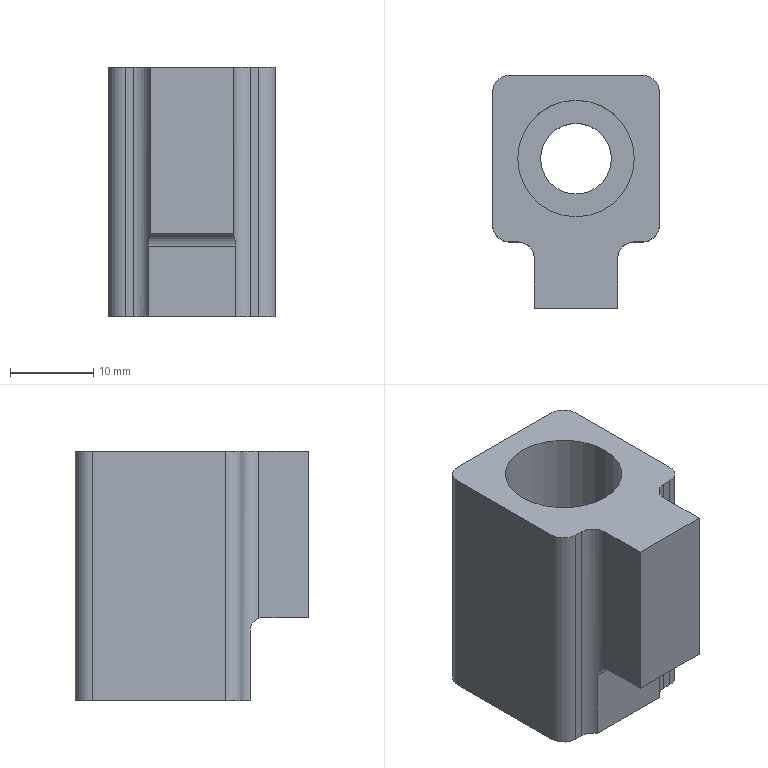Part | NX | features 1605030666 2 | 1 solid | 22 faces | box 20 x 28 x 30 mm | volume 10977 mm3 | plane 13 | cylinder 9 | commonest cylinder face diameters 4 x6 3 x1 8.5 x1 14 x1
STEP:
#1=CARTESIAN_POINT('',(-255.268,122.2,-31.5));
#2=VERTEX_POINT('',#1);
#3=CARTESIAN_POINT('',(-255.268,122.2,-23.));
#4=VERTEX_POINT('',#3);
#5=CARTESIAN_POINT('',(-255.268,122.2,-9.5));
#6=DIRECTION('',(0.,0.,-1.));
#7=VECTOR('',#6,1000.);
#8=LINE('',#5,#7);
#9=EDGE_CURVE('',#2,#4,#8,.F.);
#10=ORIENTED_EDGE('',*,*,#9,.F.);
#11=CARTESIAN_POINT('',(-244.732,122.2,-31.5));
#12=VERTEX_POINT('',#11);
#13=CARTESIAN_POINT('',(40.,122.2,-31.5));
#14=DIRECTION('',(-1.,0.,0.));
#15=VECTOR('',#14,1000.);
#16=LINE('',#13,#15);
#17=EDGE_CURVE('',#2,#12,#16,.F.);
#18=ORIENTED_EDGE('',*,*,#17,.T.);
#19=CARTESIAN_POINT('',(-244.732,122.2,-23.));
#20=VERTEX_POINT('',#19);
#21=CARTESIAN_POINT('',(-244.732,122.2,-1.5));
#22=DIRECTION('',(0.,0.,-1.));
#23=VECTOR('',#22,1000.);
#24=LINE('',#21,#23);
#25=EDGE_CURVE('',#20,#12,#24,.T.);
#26=ORIENTED_EDGE('',*,*,#25,.F.);
#27=CARTESIAN_POINT('',(-250.,122.2,-23.));
#28=DIRECTION('',(-1.,0.,0.));
#29=VECTOR('',#28,1000.);
#30=LINE('',#27,#29);
#31=EDGE_CURVE('',#4,#20,#30,.F.);
#32=ORIENTED_EDGE('',*,*,#31,.F.);
#33=EDGE_LOOP('',(#10,#18,#26,#32));
#34=FACE_BOUND('',#33,.T.);
#35=CARTESIAN_POINT('',(-250.,122.2,-76.5));
#36=DIRECTION('',(0.,1.,0.));
#37=DIRECTION('',(0.,0.,-1.));
#38=AXIS2_PLACEMENT_3D('',#35,#36,#37);
#39=PLANE('',#38);
#40=ADVANCED_FACE('',(#34),#39,.F.);
#41=ORIENTED_EDGE('',*,*,#17,.F.);
#42=CARTESIAN_POINT('',(-257.,123.2,-31.5));
#43=VERTEX_POINT('',#42);
#44=CARTESIAN_POINT('',(-257.,121.2,-31.5));
#45=DIRECTION('',(0.,0.,1.));
#46=DIRECTION('',(-1.,0.,0.));
#47=AXIS2_PLACEMENT_3D('',#44,#45,#46);
#48=CIRCLE('',#47,2.);
#49=EDGE_CURVE('',#43,#2,#48,.F.);
#50=ORIENTED_EDGE('',*,*,#49,.F.);
#51=CARTESIAN_POINT('',(-258.,123.2,-31.5));
#52=VERTEX_POINT('',#51);
#53=CARTESIAN_POINT('',(-256.,123.2,-31.5));
#54=DIRECTION('',(-1.,0.,0.));
#55=VECTOR('',#54,1000.);
#56=LINE('',#53,#55);
#57=EDGE_CURVE('',#43,#52,#56,.T.);
#58=ORIENTED_EDGE('',*,*,#57,.T.);
#59=CARTESIAN_POINT('',(-260.,125.2,-31.5));
#60=VERTEX_POINT('',#59);
#61=CARTESIAN_POINT('',(-258.,125.2,-31.5));
#62=DIRECTION('',(0.,0.,1.));
#63=DIRECTION('',(-1.,0.,0.));
#64=AXIS2_PLACEMENT_3D('',#61,#62,#63);
#65=CIRCLE('',#64,2.);
#66=EDGE_CURVE('',#60,#52,#65,.T.);
#67=ORIENTED_EDGE('',*,*,#66,.F.);
#68=CARTESIAN_POINT('',(-260.,141.2,-31.5));
#69=VERTEX_POINT('',#68);
#70=CARTESIAN_POINT('',(-260.,129.2,-31.5));
#71=DIRECTION('',(0.,1.,0.));
#72=VECTOR('',#71,1000.);
#73=LINE('',#70,#72);
#74=EDGE_CURVE('',#60,#69,#73,.T.);
#75=ORIENTED_EDGE('',*,*,#74,.T.);
#76=CARTESIAN_POINT('',(-258.,143.2,-31.5));
#77=VERTEX_POINT('',#76);
#78=CARTESIAN_POINT('',(-258.,141.2,-31.5));
#79=DIRECTION('',(0.,0.,1.));
#80=DIRECTION('',(-1.,0.,0.));
#81=AXIS2_PLACEMENT_3D('',#78,#79,#80);
#82=CIRCLE('',#81,2.);
#83=EDGE_CURVE('',#77,#69,#82,.T.);
#84=ORIENTED_EDGE('',*,*,#83,.F.);
#85=CARTESIAN_POINT('',(-242.,143.2,-31.5));
#86=VERTEX_POINT('',#85);
#87=CARTESIAN_POINT('',(-256.,143.2,-31.5));
#88=DIRECTION('',(1.,0.,0.));
#89=VECTOR('',#88,1000.);
#90=LINE('',#87,#89);
#91=EDGE_CURVE('',#77,#86,#90,.T.);
#92=ORIENTED_EDGE('',*,*,#91,.T.);
#93=CARTESIAN_POINT('',(-240.,141.2,-31.5));
#94=VERTEX_POINT('',#93);
#95=CARTESIAN_POINT('',(-242.,141.2,-31.5));
#96=DIRECTION('',(0.,0.,1.));
#97=DIRECTION('',(-1.,0.,0.));
#98=AXIS2_PLACEMENT_3D('',#95,#96,#97);
#99=CIRCLE('',#98,2.);
#100=EDGE_CURVE('',#94,#86,#99,.T.);
#101=ORIENTED_EDGE('',*,*,#100,.F.);
#102=CARTESIAN_POINT('',(-240.,125.2,-31.5));
#103=VERTEX_POINT('',#102);
#104=CARTESIAN_POINT('',(-240.,129.2,-31.5));
#105=DIRECTION('',(0.,-1.,0.));
#106=VECTOR('',#105,1000.);
#107=LINE('',#104,#106);
#108=EDGE_CURVE('',#94,#103,#107,.T.);
#109=ORIENTED_EDGE('',*,*,#108,.T.);
#110=CARTESIAN_POINT('',(-242.,123.2,-31.5));
#111=VERTEX_POINT('',#110);
#112=CARTESIAN_POINT('',(-242.,125.2,-31.5));
#113=DIRECTION('',(0.,0.,1.));
#114=DIRECTION('',(-1.,0.,0.));
#115=AXIS2_PLACEMENT_3D('',#112,#113,#114);
#116=CIRCLE('',#115,2.);
#117=EDGE_CURVE('',#111,#103,#116,.T.);
#118=ORIENTED_EDGE('',*,*,#117,.F.);
#119=CARTESIAN_POINT('',(-243.,123.2,-31.5));
#120=VERTEX_POINT('',#119);
#121=CARTESIAN_POINT('',(-256.,123.2,-31.5));
#122=DIRECTION('',(-1.,0.,0.));
#123=VECTOR('',#122,1000.);
#124=LINE('',#121,#123);
#125=EDGE_CURVE('',#111,#120,#124,.T.);
#126=ORIENTED_EDGE('',*,*,#125,.T.);
#127=CARTESIAN_POINT('',(-243.,121.2,-31.5));
#128=DIRECTION('',(0.,0.,1.));
#129=DIRECTION('',(-1.,0.,0.));
#130=AXIS2_PLACEMENT_3D('',#127,#128,#129);
#131=CIRCLE('',#130,2.);
#132=EDGE_CURVE('',#12,#120,#131,.F.);
#133=ORIENTED_EDGE('',*,*,#132,.F.);
#134=EDGE_LOOP('',(#41,#50,#58,#67,#75,#84,#92,#101,#109,#118,#126,#133));
#135=FACE_BOUND('',#134,.T.);
#136=CARTESIAN_POINT('',(-254.25,133.2,-31.5));
#137=VERTEX_POINT('',#136);
#138=CARTESIAN_POINT('',(-250.,133.2,-31.5));
#139=DIRECTION('',(0.,0.,-1.));
#140=DIRECTION('',(-1.,0.,0.));
#141=AXIS2_PLACEMENT_3D('',#138,#139,#140);
#142=CIRCLE('',#141,4.25);
#143=EDGE_CURVE('',#137,#137,#142,.T.);
#144=ORIENTED_EDGE('',*,*,#143,.F.);
#145=EDGE_LOOP('',(#144));
#146=FACE_BOUND('',#145,.T.);
#147=CARTESIAN_POINT('',(40.,31.936,-31.5));
#148=DIRECTION('',(0.,0.,-1.));
#149=DIRECTION('',(-1.,0.,0.));
#150=AXIS2_PLACEMENT_3D('',#147,#148,#149);
#151=PLANE('',#150);
#152=ADVANCED_FACE('',(#135,#146),#151,.T.);
#153=CARTESIAN_POINT('',(-243.,123.2,-1.5));
#154=VERTEX_POINT('',#153);
#155=CARTESIAN_POINT('',(-245.,121.2,-1.5));
#156=VERTEX_POINT('',#155);
#157=CARTESIAN_POINT('',(-243.,121.2,-1.5));
#158=DIRECTION('',(0.,0.,-1.));
#159=DIRECTION('',(1.,0.,0.));
#160=AXIS2_PLACEMENT_3D('',#157,#158,#159);
#161=CIRCLE('',#160,2.);
#162=EDGE_CURVE('',#154,#156,#161,.F.);
#163=ORIENTED_EDGE('',*,*,#162,.F.);
#164=CARTESIAN_POINT('',(-242.,123.2,-1.5));
#165=VERTEX_POINT('',#164);
#166=CARTESIAN_POINT('',(-256.,123.2,-1.5));
#167=DIRECTION('',(1.,0.,0.));
#168=VECTOR('',#167,1000.);
#169=LINE('',#166,#168);
#170=EDGE_CURVE('',#154,#165,#169,.T.);
#171=ORIENTED_EDGE('',*,*,#170,.T.);
#172=CARTESIAN_POINT('',(-240.,125.2,-1.5));
#173=VERTEX_POINT('',#172);
#174=CARTESIAN_POINT('',(-242.,125.2,-1.5));
#175=DIRECTION('',(0.,0.,-1.));
#176=DIRECTION('',(1.,0.,0.));
#177=AXIS2_PLACEMENT_3D('',#174,#175,#176);
#178=CIRCLE('',#177,2.);
#179=EDGE_CURVE('',#173,#165,#178,.T.);
#180=ORIENTED_EDGE('',*,*,#179,.F.);
#181=CARTESIAN_POINT('',(-240.,141.2,-1.5));
#182=VERTEX_POINT('',#181);
#183=CARTESIAN_POINT('',(-240.,129.2,-1.5));
#184=DIRECTION('',(0.,1.,0.));
#185=VECTOR('',#184,1000.);
#186=LINE('',#183,#185);
#187=EDGE_CURVE('',#173,#182,#186,.T.);
#188=ORIENTED_EDGE('',*,*,#187,.T.);
#189=CARTESIAN_POINT('',(-242.,143.2,-1.5));
#190=VERTEX_POINT('',#189);
#191=CARTESIAN_POINT('',(-242.,141.2,-1.5));
#192=DIRECTION('',(0.,0.,-1.));
#193=DIRECTION('',(1.,0.,0.));
#194=AXIS2_PLACEMENT_3D('',#191,#192,#193);
#195=CIRCLE('',#194,2.);
#196=EDGE_CURVE('',#190,#182,#195,.T.);
#197=ORIENTED_EDGE('',*,*,#196,.F.);
#198=CARTESIAN_POINT('',(-258.,143.2,-1.5));
#199=VERTEX_POINT('',#198);
#200=CARTESIAN_POINT('',(-256.,143.2,-1.5));
#201=DIRECTION('',(-1.,0.,0.));
#202=VECTOR('',#201,1000.);
#203=LINE('',#200,#202);
#204=EDGE_CURVE('',#190,#199,#203,.T.);
#205=ORIENTED_EDGE('',*,*,#204,.T.);
#206=CARTESIAN_POINT('',(-260.,141.2,-1.5));
#207=VERTEX_POINT('',#206);
#208=CARTESIAN_POINT('',(-258.,141.2,-1.5));
#209=DIRECTION('',(0.,0.,-1.));
#210=DIRECTION('',(1.,0.,0.));
#211=AXIS2_PLACEMENT_3D('',#208,#209,#210);
#212=CIRCLE('',#211,2.);
#213=EDGE_CURVE('',#207,#199,#212,.T.);
#214=ORIENTED_EDGE('',*,*,#213,.F.);
#215=CARTESIAN_POINT('',(-260.,125.2,-1.5));
#216=VERTEX_POINT('',#215);
#217=CARTESIAN_POINT('',(-260.,129.2,-1.5));
#218=DIRECTION('',(0.,-1.,0.));
#219=VECTOR('',#218,1000.);
#220=LINE('',#217,#219);
#221=EDGE_CURVE('',#207,#216,#220,.T.);
#222=ORIENTED_EDGE('',*,*,#221,.T.);
#223=CARTESIAN_POINT('',(-258.,123.2,-1.5));
#224=VERTEX_POINT('',#223);
#225=CARTESIAN_POINT('',(-258.,125.2,-1.5));
#226=DIRECTION('',(0.,0.,-1.));
#227=DIRECTION('',(1.,0.,0.));
#228=AXIS2_PLACEMENT_3D('',#225,#226,#227);
#229=CIRCLE('',#228,2.);
#230=EDGE_CURVE('',#224,#216,#229,.T.);
#231=ORIENTED_EDGE('',*,*,#230,.F.);
#232=CARTESIAN_POINT('',(-257.,123.2,-1.5));
#233=VERTEX_POINT('',#232);
#234=CARTESIAN_POINT('',(-256.,123.2,-1.5));
#235=DIRECTION('',(1.,0.,0.));
#236=VECTOR('',#235,1000.);
#237=LINE('',#234,#236);
#238=EDGE_CURVE('',#224,#233,#237,.T.);
#239=ORIENTED_EDGE('',*,*,#238,.T.);
#240=CARTESIAN_POINT('',(-255.,121.2,-1.5));
#241=VERTEX_POINT('',#240);
#242=CARTESIAN_POINT('',(-257.,121.2,-1.5));
#243=DIRECTION('',(0.,0.,-1.));
#244=DIRECTION('',(1.,0.,0.));
#245=AXIS2_PLACEMENT_3D('',#242,#243,#244);
#246=CIRCLE('',#245,2.);
#247=EDGE_CURVE('',#241,#233,#246,.F.);
#248=ORIENTED_EDGE('',*,*,#247,.F.);
#249=CARTESIAN_POINT('',(-255.,115.2,-1.5));
#250=VERTEX_POINT('',#249);
#251=CARTESIAN_POINT('',(-255.,117.7,-1.5));
#252=DIRECTION('',(0.,-1.,0.));
#253=VECTOR('',#252,1000.);
#254=LINE('',#251,#253);
#255=EDGE_CURVE('',#241,#250,#254,.T.);
#256=ORIENTED_EDGE('',*,*,#255,.T.);
#257=CARTESIAN_POINT('',(-245.,115.2,-1.5));
#258=VERTEX_POINT('',#257);
#259=CARTESIAN_POINT('',(-250.,115.2,-1.5));
#260=DIRECTION('',(1.,0.,0.));
#261=VECTOR('',#260,1000.);
#262=LINE('',#259,#261);
#263=EDGE_CURVE('',#250,#258,#262,.T.);
#264=ORIENTED_EDGE('',*,*,#263,.T.);
#265=CARTESIAN_POINT('',(-245.,117.7,-1.5));
#266=DIRECTION('',(0.,1.,0.));
#267=VECTOR('',#266,1000.);
#268=LINE('',#265,#267);
#269=EDGE_CURVE('',#258,#156,#268,.T.);
#270=ORIENTED_EDGE('',*,*,#269,.T.);
#271=EDGE_LOOP('',(#163,#171,#180,#188,#197,#205,#214,#222,#231,#239,#248,#256,#264,#270));
#272=FACE_BOUND('',#271,.T.);
#273=CARTESIAN_POINT('',(-243.,133.2,-1.5));
#274=VERTEX_POINT('',#273);
#275=CARTESIAN_POINT('',(-250.,133.2,-1.5));
#276=DIRECTION('',(0.,0.,1.));
#277=DIRECTION('',(1.,0.,0.));
#278=AXIS2_PLACEMENT_3D('',#275,#276,#277);
#279=CIRCLE('',#278,7.);
#280=EDGE_CURVE('',#274,#274,#279,.F.);
#281=ORIENTED_EDGE('',*,*,#280,.T.);
#282=EDGE_LOOP('',(#281));
#283=FACE_BOUND('',#282,.T.);
#284=CARTESIAN_POINT('',(-250.,117.7,-1.5));
#285=DIRECTION('',(0.,0.,1.));
#286=DIRECTION('',(1.,0.,0.));
#287=AXIS2_PLACEMENT_3D('',#284,#285,#286);
#288=PLANE('',#287);
#289=ADVANCED_FACE('',(#272,#283),#288,.T.);
#290=ORIENTED_EDGE('',*,*,#238,.F.);
#291=CARTESIAN_POINT('',(-258.,123.2,-1.5));
#292=DIRECTION('',(0.,0.,-1.));
#293=VECTOR('',#292,1000.);
#294=LINE('',#291,#293);
#295=EDGE_CURVE('',#52,#224,#294,.F.);
#296=ORIENTED_EDGE('',*,*,#295,.F.);
#297=ORIENTED_EDGE('',*,*,#57,.F.);
#298=CARTESIAN_POINT('',(-257.,123.2,-36.5));
#299=DIRECTION('',(0.,0.,1.));
#300=VECTOR('',#299,1000.);
#301=LINE('',#298,#300);
#302=EDGE_CURVE('',#233,#43,#301,.F.);
#303=ORIENTED_EDGE('',*,*,#302,.F.);
#304=EDGE_LOOP('',(#290,#296,#297,#303));
#305=FACE_BOUND('',#304,.T.);
#306=CARTESIAN_POINT('',(-256.,123.2,-1.5));
#307=DIRECTION('',(0.,-1.,0.));
#308=DIRECTION('',(0.,0.,1.));
#309=AXIS2_PLACEMENT_3D('',#306,#307,#308);
#310=PLANE('',#309);
#311=ADVANCED_FACE('',(#305),#310,.T.);
#312=ORIENTED_EDGE('',*,*,#91,.F.);
#313=CARTESIAN_POINT('',(-258.,143.2,-1.5));
#314=DIRECTION('',(0.,0.,-1.));
#315=VECTOR('',#314,1000.);
#316=LINE('',#313,#315);
#317=EDGE_CURVE('',#199,#77,#316,.T.);
#318=ORIENTED_EDGE('',*,*,#317,.F.);
#319=ORIENTED_EDGE('',*,*,#204,.F.);
#320=CARTESIAN_POINT('',(-242.,143.2,-1.5));
#321=DIRECTION('',(0.,0.,-1.));
#322=VECTOR('',#321,1000.);
#323=LINE('',#320,#322);
#324=EDGE_CURVE('',#86,#190,#323,.F.);
#325=ORIENTED_EDGE('',*,*,#324,.F.);
#326=EDGE_LOOP('',(#312,#318,#319,#325));
#327=FACE_BOUND('',#326,.T.);
#328=CARTESIAN_POINT('',(-256.,143.2,-1.5));
#329=DIRECTION('',(0.,1.,0.));
#330=DIRECTION('',(0.,0.,-1.));
#331=AXIS2_PLACEMENT_3D('',#328,#329,#330);
#332=PLANE('',#331);
#333=ADVANCED_FACE('',(#327),#332,.T.);
#334=ORIENTED_EDGE('',*,*,#108,.F.);
#335=CARTESIAN_POINT('',(-240.,141.2,-1.5));
#336=DIRECTION('',(0.,0.,-1.));
#337=VECTOR('',#336,1000.);
#338=LINE('',#335,#337);
#339=EDGE_CURVE('',#182,#94,#338,.T.);
#340=ORIENTED_EDGE('',*,*,#339,.F.);
#341=ORIENTED_EDGE('',*,*,#187,.F.);
#342=CARTESIAN_POINT('',(-240.,125.2,-1.5));
#343=DIRECTION('',(0.,0.,-1.));
#344=VECTOR('',#343,1000.);
#345=LINE('',#342,#344);
#346=EDGE_CURVE('',#103,#173,#345,.F.);
#347=ORIENTED_EDGE('',*,*,#346,.F.);
#348=EDGE_LOOP('',(#334,#340,#341,#347));
#349=FACE_BOUND('',#348,.T.);
#350=CARTESIAN_POINT('',(-240.,129.2,-1.5));
#351=DIRECTION('',(1.,0.,0.));
#352=DIRECTION('',(0.,0.,-1.));
#353=AXIS2_PLACEMENT_3D('',#350,#351,#352);
#354=PLANE('',#353);
#355=ADVANCED_FACE('',(#349),#354,.T.);
#356=ORIENTED_EDGE('',*,*,#125,.F.);
#357=CARTESIAN_POINT('',(-242.,123.2,-1.5));
#358=DIRECTION('',(0.,0.,-1.));
#359=VECTOR('',#358,1000.);
#360=LINE('',#357,#359);
#361=EDGE_CURVE('',#165,#111,#360,.T.);
#362=ORIENTED_EDGE('',*,*,#361,.F.);
#363=ORIENTED_EDGE('',*,*,#170,.F.);
#364=CARTESIAN_POINT('',(-243.,123.2,-1.5));
#365=DIRECTION('',(0.,0.,1.));
#366=VECTOR('',#365,1000.);
#367=LINE('',#364,#366);
#368=EDGE_CURVE('',#120,#154,#367,.T.);
#369=ORIENTED_EDGE('',*,*,#368,.F.);
#370=EDGE_LOOP('',(#356,#362,#363,#369));
#371=FACE_BOUND('',#370,.T.);
#372=CARTESIAN_POINT('',(-256.,123.2,-1.5));
#373=DIRECTION('',(0.,-1.,0.));
#374=DIRECTION('',(0.,0.,1.));
#375=AXIS2_PLACEMENT_3D('',#372,#373,#374);
#376=PLANE('',#375);
#377=ADVANCED_FACE('',(#371),#376,.T.);
#378=ORIENTED_EDGE('',*,*,#221,.F.);
#379=CARTESIAN_POINT('',(-260.,141.2,-1.5));
#380=DIRECTION('',(0.,0.,-1.));
#381=VECTOR('',#380,1000.);
#382=LINE('',#379,#381);
#383=EDGE_CURVE('',#69,#207,#382,.F.);
#384=ORIENTED_EDGE('',*,*,#383,.F.);
#385=ORIENTED_EDGE('',*,*,#74,.F.);
#386=CARTESIAN_POINT('',(-260.,125.2,-1.5));
#387=DIRECTION('',(0.,0.,-1.));
#388=VECTOR('',#387,1000.);
#389=LINE('',#386,#388);
#390=EDGE_CURVE('',#216,#60,#389,.T.);
#391=ORIENTED_EDGE('',*,*,#390,.F.);
#392=EDGE_LOOP('',(#378,#384,#385,#391));
#393=FACE_BOUND('',#392,.T.);
#394=CARTESIAN_POINT('',(-260.,129.2,-1.5));
#395=DIRECTION('',(-1.,0.,0.));
#396=DIRECTION('',(0.,0.,1.));
#397=AXIS2_PLACEMENT_3D('',#394,#395,#396);
#398=PLANE('',#397);
#399=ADVANCED_FACE('',(#393),#398,.T.);
#400=ORIENTED_EDGE('',*,*,#213,.T.);
#401=ORIENTED_EDGE('',*,*,#317,.T.);
#402=ORIENTED_EDGE('',*,*,#83,.T.);
#403=ORIENTED_EDGE('',*,*,#383,.T.);
#404=EDGE_LOOP('',(#400,#401,#402,#403));
#405=FACE_BOUND('',#404,.T.);
#406=CARTESIAN_POINT('',(-258.,141.2,-1.5));
#407=DIRECTION('',(0.,0.,-1.));
#408=DIRECTION('',(-1.,0.,0.));
#409=AXIS2_PLACEMENT_3D('',#406,#407,#408);
#410=CYLINDRICAL_SURFACE('',#409,2.);
#411=ADVANCED_FACE('',(#405),#410,.T.);
#412=ORIENTED_EDGE('',*,*,#196,.T.);
#413=ORIENTED_EDGE('',*,*,#339,.T.);
#414=ORIENTED_EDGE('',*,*,#100,.T.);
#415=ORIENTED_EDGE('',*,*,#324,.T.);
#416=EDGE_LOOP('',(#412,#413,#414,#415));
#417=FACE_BOUND('',#416,.T.);
#418=CARTESIAN_POINT('',(-242.,141.2,-1.5));
#419=DIRECTION('',(0.,0.,-1.));
#420=DIRECTION('',(-1.,0.,0.));
#421=AXIS2_PLACEMENT_3D('',#418,#419,#420);
#422=CYLINDRICAL_SURFACE('',#421,2.);
#423=ADVANCED_FACE('',(#417),#422,.T.);
#424=ORIENTED_EDGE('',*,*,#179,.T.);
#425=ORIENTED_EDGE('',*,*,#361,.T.);
#426=ORIENTED_EDGE('',*,*,#117,.T.);
#427=ORIENTED_EDGE('',*,*,#346,.T.);
#428=EDGE_LOOP('',(#424,#425,#426,#427));
#429=FACE_BOUND('',#428,.T.);
#430=CARTESIAN_POINT('',(-242.,125.2,-1.5));
#431=DIRECTION('',(0.,0.,-1.));
#432=DIRECTION('',(-1.,0.,0.));
#433=AXIS2_PLACEMENT_3D('',#430,#431,#432);
#434=CYLINDRICAL_SURFACE('',#433,2.);
#435=ADVANCED_FACE('',(#429),#434,.T.);
#436=ORIENTED_EDGE('',*,*,#230,.T.);
#437=ORIENTED_EDGE('',*,*,#390,.T.);
#438=ORIENTED_EDGE('',*,*,#66,.T.);
#439=ORIENTED_EDGE('',*,*,#295,.T.);
#440=EDGE_LOOP('',(#436,#437,#438,#439));
#441=FACE_BOUND('',#440,.T.);
#442=CARTESIAN_POINT('',(-258.,125.2,-1.5));
#443=DIRECTION('',(0.,0.,-1.));
#444=DIRECTION('',(-1.,0.,0.));
#445=AXIS2_PLACEMENT_3D('',#442,#443,#444);
#446=CYLINDRICAL_SURFACE('',#445,2.);
#447=ADVANCED_FACE('',(#441),#446,.T.);
#448=ORIENTED_EDGE('',*,*,#49,.T.);
#449=ORIENTED_EDGE('',*,*,#9,.T.);
#450=CARTESIAN_POINT('',(-255.,121.2,-21.586));
#451=VERTEX_POINT('',#450);
#452=CARTESIAN_POINT('',(-255.,121.2,-21.586));
#453=CARTESIAN_POINT('',(-255.,121.794,-21.796));
#454=CARTESIAN_POINT('',(-255.268,122.2,-22.37));
#455=CARTESIAN_POINT('',(-255.268,122.2,-23.));
#456=B_SPLINE_CURVE_WITH_KNOTS('',3,(#452,#453,#454,#455),.UNSPECIFIED.,.F.,.F.,(4,4),(0.,0.001858),.UNSPECIFIED.);
#457=EDGE_CURVE('',#451,#4,#456,.T.);
#458=ORIENTED_EDGE('',*,*,#457,.F.);
#459=CARTESIAN_POINT('',(-255.,121.2,-9.5));
#460=DIRECTION('',(0.,0.,-1.));
#461=VECTOR('',#460,1000.);
#462=LINE('',#459,#461);
#463=EDGE_CURVE('',#451,#241,#462,.F.);
#464=ORIENTED_EDGE('',*,*,#463,.T.);
#465=ORIENTED_EDGE('',*,*,#247,.T.);
#466=ORIENTED_EDGE('',*,*,#302,.T.);
#467=EDGE_LOOP('',(#448,#449,#458,#464,#465,#466));
#468=FACE_BOUND('',#467,.T.);
#469=CARTESIAN_POINT('',(-257.,121.2,-9.5));
#470=DIRECTION('',(0.,0.,-1.));
#471=DIRECTION('',(-1.,0.,0.));
#472=AXIS2_PLACEMENT_3D('',#469,#470,#471);
#473=CYLINDRICAL_SURFACE('',#472,2.);
#474=ADVANCED_FACE('',(#468),#473,.F.);
#475=ORIENTED_EDGE('',*,*,#132,.T.);
#476=ORIENTED_EDGE('',*,*,#368,.T.);
#477=ORIENTED_EDGE('',*,*,#162,.T.);
#478=CARTESIAN_POINT('',(-245.,121.2,-21.586));
#479=VERTEX_POINT('',#478);
#480=CARTESIAN_POINT('',(-245.,121.2,-36.5));
#481=DIRECTION('',(0.,0.,1.));
#482=VECTOR('',#481,1000.);
#483=LINE('',#480,#482);
#484=EDGE_CURVE('',#156,#479,#483,.F.);
#485=ORIENTED_EDGE('',*,*,#484,.T.);
#486=CARTESIAN_POINT('',(-244.732,122.2,-23.));
#487=CARTESIAN_POINT('',(-244.732,122.2,-22.37));
#488=CARTESIAN_POINT('',(-245.,121.794,-21.796));
#489=CARTESIAN_POINT('',(-245.,121.2,-21.586));
#490=B_SPLINE_CURVE_WITH_KNOTS('',3,(#486,#487,#488,#489),.UNSPECIFIED.,.F.,.F.,(4,4),(0.,0.001858),.UNSPECIFIED.);
#491=EDGE_CURVE('',#20,#479,#490,.T.);
#492=ORIENTED_EDGE('',*,*,#491,.F.);
#493=ORIENTED_EDGE('',*,*,#25,.T.);
#494=EDGE_LOOP('',(#475,#476,#477,#485,#492,#493));
#495=FACE_BOUND('',#494,.T.);
#496=CARTESIAN_POINT('',(-243.,121.2,-1.5));
#497=DIRECTION('',(0.,0.,-1.));
#498=DIRECTION('',(-1.,0.,0.));
#499=AXIS2_PLACEMENT_3D('',#496,#497,#498);
#500=CYLINDRICAL_SURFACE('',#499,2.);
#501=ADVANCED_FACE('',(#495),#500,.F.);
#502=CARTESIAN_POINT('',(-254.25,133.2,-11.5));
#503=VERTEX_POINT('',#502);
#504=CARTESIAN_POINT('',(-250.,133.2,-11.5));
#505=DIRECTION('',(0.,0.,-1.));
#506=DIRECTION('',(-1.,0.,0.));
#507=AXIS2_PLACEMENT_3D('',#504,#505,#506);
#508=CIRCLE('',#507,4.25);
#509=EDGE_CURVE('',#503,#503,#508,.T.);
#510=ORIENTED_EDGE('',*,*,#509,.F.);
#511=EDGE_LOOP('',(#510));
#512=FACE_BOUND('',#511,.T.);
#513=ORIENTED_EDGE('',*,*,#143,.T.);
#514=EDGE_LOOP('',(#513));
#515=FACE_BOUND('',#514,.T.);
#516=CARTESIAN_POINT('',(-250.,133.2,-31.5));
#517=DIRECTION('',(0.,0.,1.));
#518=DIRECTION('',(1.,0.,0.));
#519=AXIS2_PLACEMENT_3D('',#516,#517,#518);
#520=CYLINDRICAL_SURFACE('',#519,4.25);
#521=ADVANCED_FACE('',(#512,#515),#520,.F.);
#522=CARTESIAN_POINT('',(-257.,133.2,-11.5));
#523=VERTEX_POINT('',#522);
#524=CARTESIAN_POINT('',(-250.,133.2,-11.5));
#525=DIRECTION('',(0.,0.,-1.));
#526=DIRECTION('',(-1.,0.,0.));
#527=AXIS2_PLACEMENT_3D('',#524,#525,#526);
#528=CIRCLE('',#527,7.);
#529=EDGE_CURVE('',#523,#523,#528,.F.);
#530=ORIENTED_EDGE('',*,*,#529,.T.);
#531=EDGE_LOOP('',(#530));
#532=FACE_BOUND('',#531,.T.);
#533=ORIENTED_EDGE('',*,*,#509,.T.);
#534=EDGE_LOOP('',(#533));
#535=FACE_BOUND('',#534,.T.);
#536=CARTESIAN_POINT('',(-250.,133.2,-11.5));
#537=DIRECTION('',(0.,0.,-1.));
#538=DIRECTION('',(-1.,0.,0.));
#539=AXIS2_PLACEMENT_3D('',#536,#537,#538);
#540=PLANE('',#539);
#541=ADVANCED_FACE('',(#532,#535),#540,.F.);
#542=ORIENTED_EDGE('',*,*,#280,.F.);
#543=EDGE_LOOP('',(#542));
#544=FACE_BOUND('',#543,.T.);
#545=ORIENTED_EDGE('',*,*,#529,.F.);
#546=EDGE_LOOP('',(#545));
#547=FACE_BOUND('',#546,.T.);
#548=CARTESIAN_POINT('',(-250.,133.2,-11.5));
#549=DIRECTION('',(0.,0.,1.));
#550=DIRECTION('',(1.,0.,0.));
#551=AXIS2_PLACEMENT_3D('',#548,#549,#550);
#552=CYLINDRICAL_SURFACE('',#551,7.);
#553=ADVANCED_FACE('',(#544,#547),#552,.F.);
#554=CARTESIAN_POINT('',(-255.,115.2,-21.5));
#555=VERTEX_POINT('',#554);
#556=CARTESIAN_POINT('',(-255.,115.2,-9.5));
#557=DIRECTION('',(0.,0.,1.));
#558=VECTOR('',#557,1000.);
#559=LINE('',#556,#558);
#560=EDGE_CURVE('',#555,#250,#559,.T.);
#561=ORIENTED_EDGE('',*,*,#560,.F.);
#562=CARTESIAN_POINT('',(-245.,115.2,-21.5));
#563=VERTEX_POINT('',#562);
#564=CARTESIAN_POINT('',(-250.,115.2,-21.5));
#565=DIRECTION('',(-1.,0.,0.));
#566=VECTOR('',#565,1000.);
#567=LINE('',#564,#566);
#568=EDGE_CURVE('',#563,#555,#567,.T.);
#569=ORIENTED_EDGE('',*,*,#568,.F.);
#570=CARTESIAN_POINT('',(-245.,115.2,-9.5));
#571=DIRECTION('',(0.,0.,1.));
#572=VECTOR('',#571,1000.);
#573=LINE('',#570,#572);
#574=EDGE_CURVE('',#563,#258,#573,.T.);
#575=ORIENTED_EDGE('',*,*,#574,.T.);
#576=ORIENTED_EDGE('',*,*,#263,.F.);
#577=EDGE_LOOP('',(#561,#569,#575,#576));
#578=FACE_BOUND('',#577,.T.);
#579=CARTESIAN_POINT('',(-250.,115.2,-9.5));
#580=DIRECTION('',(0.,-1.,0.));
#581=DIRECTION('',(0.,0.,1.));
#582=AXIS2_PLACEMENT_3D('',#579,#580,#581);
#583=PLANE('',#582);
#584=ADVANCED_FACE('',(#578),#583,.T.);
#585=ORIENTED_EDGE('',*,*,#269,.F.);
#586=ORIENTED_EDGE('',*,*,#574,.F.);
#587=CARTESIAN_POINT('',(-245.,120.7,-21.5));
#588=VERTEX_POINT('',#587);
#589=CARTESIAN_POINT('',(-245.,117.7,-21.5));
#590=DIRECTION('',(0.,-1.,0.));
#591=VECTOR('',#590,1000.);
#592=LINE('',#589,#591);
#593=EDGE_CURVE('',#588,#563,#592,.T.);
#594=ORIENTED_EDGE('',*,*,#593,.F.);
#595=CARTESIAN_POINT('',(-245.,120.7,-23.));
#596=DIRECTION('',(-1.,0.,0.));
#597=DIRECTION('',(0.,0.,-1.));
#598=AXIS2_PLACEMENT_3D('',#595,#596,#597);
#599=CIRCLE('',#598,1.5);
#600=EDGE_CURVE('',#479,#588,#599,.F.);
#601=ORIENTED_EDGE('',*,*,#600,.F.);
#602=ORIENTED_EDGE('',*,*,#484,.F.);
#603=EDGE_LOOP('',(#585,#586,#594,#601,#602));
#604=FACE_BOUND('',#603,.T.);
#605=CARTESIAN_POINT('',(-245.,117.7,-9.5));
#606=DIRECTION('',(1.,0.,0.));
#607=DIRECTION('',(0.,0.,-1.));
#608=AXIS2_PLACEMENT_3D('',#605,#606,#607);
#609=PLANE('',#608);
#610=ADVANCED_FACE('',(#604),#609,.T.);
#611=CARTESIAN_POINT('',(-255.,120.7,-21.5));
#612=VERTEX_POINT('',#611);
#613=CARTESIAN_POINT('',(-255.,117.7,-21.5));
#614=DIRECTION('',(0.,1.,0.));
#615=VECTOR('',#614,1000.);
#616=LINE('',#613,#615);
#617=EDGE_CURVE('',#555,#612,#616,.T.);
#618=ORIENTED_EDGE('',*,*,#617,.F.);
#619=ORIENTED_EDGE('',*,*,#560,.T.);
#620=ORIENTED_EDGE('',*,*,#255,.F.);
#621=ORIENTED_EDGE('',*,*,#463,.F.);
#622=CARTESIAN_POINT('',(-255.,120.7,-23.));
#623=DIRECTION('',(1.,0.,0.));
#624=DIRECTION('',(0.,0.,1.));
#625=AXIS2_PLACEMENT_3D('',#622,#623,#624);
#626=CIRCLE('',#625,1.5);
#627=EDGE_CURVE('',#612,#451,#626,.F.);
#628=ORIENTED_EDGE('',*,*,#627,.F.);
#629=EDGE_LOOP('',(#618,#619,#620,#621,#628));
#630=FACE_BOUND('',#629,.T.);
#631=CARTESIAN_POINT('',(-255.,117.7,-9.5));
#632=DIRECTION('',(-1.,0.,0.));
#633=DIRECTION('',(0.,0.,1.));
#634=AXIS2_PLACEMENT_3D('',#631,#632,#633);
#635=PLANE('',#634);
#636=ADVANCED_FACE('',(#630),#635,.T.);
#637=ORIENTED_EDGE('',*,*,#593,.T.);
#638=ORIENTED_EDGE('',*,*,#568,.T.);
#639=ORIENTED_EDGE('',*,*,#617,.T.);
#640=CARTESIAN_POINT('',(40.,120.7,-21.5));
#641=DIRECTION('',(-1.,0.,0.));
#642=VECTOR('',#641,1000.);
#643=LINE('',#640,#642);
#644=EDGE_CURVE('',#588,#612,#643,.T.);
#645=ORIENTED_EDGE('',*,*,#644,.F.);
#646=EDGE_LOOP('',(#637,#638,#639,#645));
#647=FACE_BOUND('',#646,.T.);
#648=CARTESIAN_POINT('',(40.,31.936,-21.5));
#649=DIRECTION('',(0.,0.,-1.));
#650=DIRECTION('',(-1.,0.,0.));
#651=AXIS2_PLACEMENT_3D('',#648,#649,#650);
#652=PLANE('',#651);
#653=ADVANCED_FACE('',(#647),#652,.T.);
#654=ORIENTED_EDGE('',*,*,#491,.T.);
#655=ORIENTED_EDGE('',*,*,#600,.T.);
#656=ORIENTED_EDGE('',*,*,#644,.T.);
#657=ORIENTED_EDGE('',*,*,#627,.T.);
#658=ORIENTED_EDGE('',*,*,#457,.T.);
#659=ORIENTED_EDGE('',*,*,#31,.T.);
#660=EDGE_LOOP('',(#654,#655,#656,#657,#658,#659));
#661=FACE_BOUND('',#660,.T.);
#662=CARTESIAN_POINT('',(40.,120.7,-23.));
#663=DIRECTION('',(-1.,0.,0.));
#664=DIRECTION('',(0.,0.,1.));
#665=AXIS2_PLACEMENT_3D('',#662,#663,#664);
#666=CYLINDRICAL_SURFACE('',#665,1.5);
#667=ADVANCED_FACE('',(#661),#666,.F.);
#668=CLOSED_SHELL('',(#40,#152,#289,#311,#333,#355,#377,#399,#411,#423,#435,#447,#474,#501,#521,#541,#553,#584,#610,#636,#653,#667));
#669=MANIFOLD_SOLID_BREP('',#668);
#670=(LENGTH_UNIT()NAMED_UNIT(*)SI_UNIT(.MILLI.,.METRE.));
#671=UNCERTAINTY_MEASURE_WITH_UNIT(LENGTH_MEASURE(0.0508),#670,'','');
#672=(NAMED_UNIT(*)PLANE_ANGLE_UNIT()SI_UNIT($,.RADIAN.));
#673=(NAMED_UNIT(*)SI_UNIT($,.STERADIAN.)SOLID_ANGLE_UNIT());
#674=(GEOMETRIC_REPRESENTATION_CONTEXT(3)GLOBAL_UNCERTAINTY_ASSIGNED_CONTEXT((#671))GLOBAL_UNIT_ASSIGNED_CONTEXT((#670,#672,#673))REPRESENTATION_CONTEXT('',''));
#675=ADVANCED_BREP_SHAPE_REPRESENTATION('',(#669),#674);